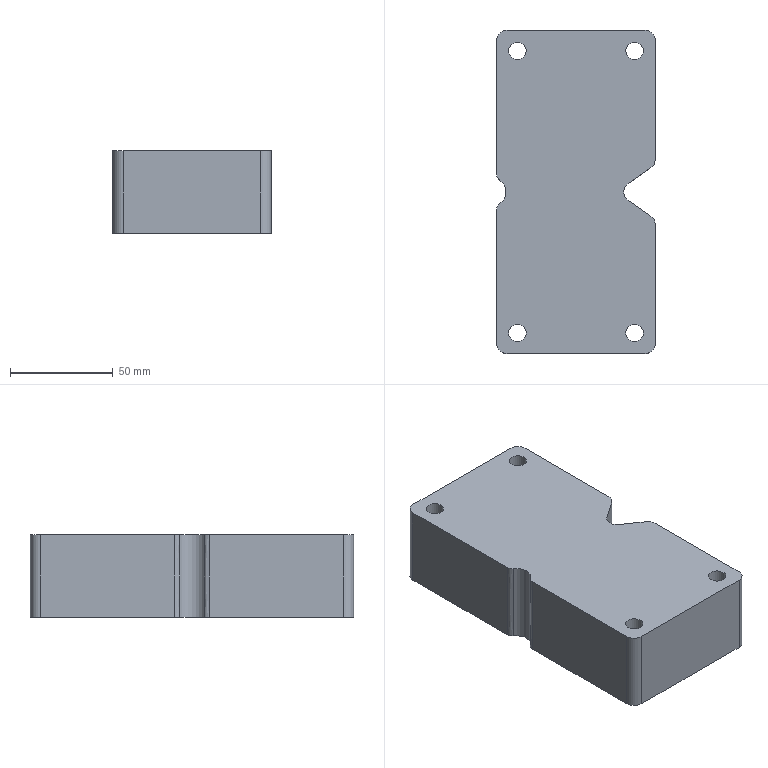Part | NX | features PS-14 2 | 1 solid | 32 faces | box 77 x 157.001 x 40 mm | volume 457397 mm3 | cylinder 16 | plane 14 | spline 2 | commonest cylinder face diameters 10 x7 8.5 x4 14.5 x4 14.05 x1
STEP:
#1=CARTESIAN_POINT('',(2764.236,-866.479,900.716));
#2=VERTEX_POINT('',#1);
#3=CARTESIAN_POINT('',(2764.236,-931.623,900.716));
#4=VERTEX_POINT('',#3);
#5=CARTESIAN_POINT('',(2764.236,-839.123,900.716));
#6=DIRECTION('',(0.,-1.,0.000000114));
#7=VECTOR('',#6,1000.);
#8=LINE('',#5,#7);
#9=EDGE_CURVE('',#2,#4,#8,.T.);
#10=ORIENTED_EDGE('',*,*,#9,.F.);
#11=CARTESIAN_POINT('',(2764.236,-866.479,860.716));
#12=VERTEX_POINT('',#11);
#13=CARTESIAN_POINT('',(2764.236,-866.479,900.716));
#14=CARTESIAN_POINT('',(2764.236,-866.479,887.383));
#15=CARTESIAN_POINT('',(2764.236,-866.479,874.05));
#16=CARTESIAN_POINT('',(2764.236,-866.479,860.716));
#17=B_SPLINE_CURVE_WITH_KNOTS('',3,(#13,#14,#15,#16),.UNSPECIFIED.,.F.,.F.,(4,4),(-0.01,0.03),.UNSPECIFIED.);
#18=EDGE_CURVE('',#2,#12,#17,.T.);
#19=ORIENTED_EDGE('',*,*,#18,.T.);
#20=CARTESIAN_POINT('',(2764.236,-896.605,860.716));
#21=VERTEX_POINT('',#20);
#22=CARTESIAN_POINT('',(2764.236,-839.123,860.716));
#23=DIRECTION('',(0.,1.,-0.000000114));
#24=VECTOR('',#23,1000.);
#25=LINE('',#22,#24);
#26=EDGE_CURVE('',#21,#12,#25,.T.);
#27=ORIENTED_EDGE('',*,*,#26,.F.);
#28=CARTESIAN_POINT('',(2764.236,-931.623,860.716));
#29=VERTEX_POINT('',#28);
#30=CARTESIAN_POINT('',(2764.236,-839.123,860.716));
#31=DIRECTION('',(0.,1.,-0.000000114));
#32=VECTOR('',#31,1000.);
#33=LINE('',#30,#32);
#34=EDGE_CURVE('',#29,#21,#33,.T.);
#35=ORIENTED_EDGE('',*,*,#34,.F.);
#36=CARTESIAN_POINT('',(2764.236,-931.623,935.716));
#37=DIRECTION('',(0.,0.,-1.));
#38=VECTOR('',#37,1000.);
#39=LINE('',#36,#38);
#40=EDGE_CURVE('',#29,#4,#39,.F.);
#41=ORIENTED_EDGE('',*,*,#40,.T.);
#42=EDGE_LOOP('',(#10,#19,#27,#35,#41));
#43=FACE_BOUND('',#42,.T.);
#44=CARTESIAN_POINT('',(2764.236,-839.123,930.716));
#45=DIRECTION('',(-1.,0.,0.));
#46=DIRECTION('',(0.,0.000000114,1.));
#47=AXIS2_PLACEMENT_3D('',#44,#45,#46);
#48=PLANE('',#47);
#49=ADVANCED_FACE('',(#43),#48,.T.);
#50=CARTESIAN_POINT('',(2769.236,-779.622,860.716));
#51=VERTEX_POINT('',#50);
#52=CARTESIAN_POINT('',(2769.236,-779.622,900.716));
#53=VERTEX_POINT('',#52);
#54=CARTESIAN_POINT('',(2769.236,-779.622,935.716));
#55=DIRECTION('',(0.,0.,-1.));
#56=VECTOR('',#55,1000.);
#57=LINE('',#54,#56);
#58=EDGE_CURVE('',#51,#53,#57,.F.);
#59=ORIENTED_EDGE('',*,*,#58,.T.);
#60=CARTESIAN_POINT('',(2836.236,-779.622,900.716));
#61=VERTEX_POINT('',#60);
#62=CARTESIAN_POINT('',(2802.736,-779.622,900.716));
#63=DIRECTION('',(-1.,0.,0.));
#64=VECTOR('',#63,1000.);
#65=LINE('',#62,#64);
#66=EDGE_CURVE('',#61,#53,#65,.T.);
#67=ORIENTED_EDGE('',*,*,#66,.F.);
#68=CARTESIAN_POINT('',(2836.236,-779.622,860.716));
#69=VERTEX_POINT('',#68);
#70=CARTESIAN_POINT('',(2836.236,-779.622,860.716));
#71=DIRECTION('',(0.,0.,-1.));
#72=VECTOR('',#71,1000.);
#73=LINE('',#70,#72);
#74=EDGE_CURVE('',#61,#69,#73,.T.);
#75=ORIENTED_EDGE('',*,*,#74,.T.);
#76=CARTESIAN_POINT('',(2798.548,-779.622,860.716));
#77=VERTEX_POINT('',#76);
#78=CARTESIAN_POINT('',(2765.986,-779.622,860.716));
#79=DIRECTION('',(1.,0.,0.));
#80=VECTOR('',#79,1000.);
#81=LINE('',#78,#80);
#82=EDGE_CURVE('',#77,#69,#81,.T.);
#83=ORIENTED_EDGE('',*,*,#82,.F.);
#84=CARTESIAN_POINT('',(2793.195,-779.622,860.716));
#85=VERTEX_POINT('',#84);
#86=CARTESIAN_POINT('',(2765.986,-779.622,860.716));
#87=DIRECTION('',(1.,0.,0.));
#88=VECTOR('',#87,1000.);
#89=LINE('',#86,#88);
#90=EDGE_CURVE('',#85,#77,#89,.T.);
#91=ORIENTED_EDGE('',*,*,#90,.F.);
#92=CARTESIAN_POINT('',(2765.986,-779.622,860.716));
#93=DIRECTION('',(1.,0.,0.));
#94=VECTOR('',#93,1000.);
#95=LINE('',#92,#94);
#96=EDGE_CURVE('',#51,#85,#95,.T.);
#97=ORIENTED_EDGE('',*,*,#96,.F.);
#98=EDGE_LOOP('',(#59,#67,#75,#83,#91,#97));
#99=FACE_BOUND('',#98,.T.);
#100=CARTESIAN_POINT('',(2765.986,-779.622,841.216));
#101=DIRECTION('',(0.,-1.,0.));
#102=DIRECTION('',(0.,0.,-1.));
#103=AXIS2_PLACEMENT_3D('',#100,#101,#102);
#104=PLANE('',#103);
#105=ADVANCED_FACE('',(#99),#104,.F.);
#106=CARTESIAN_POINT('',(2764.236,-849.765,860.716));
#107=VERTEX_POINT('',#106);
#108=CARTESIAN_POINT('',(2764.236,-819.639,860.716));
#109=VERTEX_POINT('',#108);
#110=CARTESIAN_POINT('',(2764.236,-839.123,860.716));
#111=DIRECTION('',(0.,1.,-0.000000114));
#112=VECTOR('',#111,1000.);
#113=LINE('',#110,#112);
#114=EDGE_CURVE('',#107,#109,#113,.T.);
#115=ORIENTED_EDGE('',*,*,#114,.F.);
#116=CARTESIAN_POINT('',(2764.236,-849.765,900.716));
#117=VERTEX_POINT('',#116);
#118=CARTESIAN_POINT('',(2764.236,-849.765,860.716));
#119=CARTESIAN_POINT('',(2764.236,-849.765,874.05));
#120=CARTESIAN_POINT('',(2764.236,-849.765,887.383));
#121=CARTESIAN_POINT('',(2764.236,-849.765,900.716));
#122=B_SPLINE_CURVE_WITH_KNOTS('',3,(#118,#119,#120,#121),.UNSPECIFIED.,.F.,.F.,(4,4),(0.,0.04),.UNSPECIFIED.);
#123=EDGE_CURVE('',#107,#117,#122,.T.);
#124=ORIENTED_EDGE('',*,*,#123,.T.);
#125=CARTESIAN_POINT('',(2764.236,-784.622,900.716));
#126=VERTEX_POINT('',#125);
#127=CARTESIAN_POINT('',(2764.236,-839.123,900.716));
#128=DIRECTION('',(0.,-1.,0.000000114));
#129=VECTOR('',#128,1000.);
#130=LINE('',#127,#129);
#131=EDGE_CURVE('',#126,#117,#130,.T.);
#132=ORIENTED_EDGE('',*,*,#131,.F.);
#133=CARTESIAN_POINT('',(2764.236,-784.622,860.716));
#134=VERTEX_POINT('',#133);
#135=CARTESIAN_POINT('',(2764.236,-784.622,860.716));
#136=DIRECTION('',(0.,0.,-1.));
#137=VECTOR('',#136,1000.);
#138=LINE('',#135,#137);
#139=EDGE_CURVE('',#126,#134,#138,.T.);
#140=ORIENTED_EDGE('',*,*,#139,.T.);
#141=CARTESIAN_POINT('',(2764.236,-839.123,860.716));
#142=DIRECTION('',(0.,1.,-0.000000114));
#143=VECTOR('',#142,1000.);
#144=LINE('',#141,#143);
#145=EDGE_CURVE('',#109,#134,#144,.T.);
#146=ORIENTED_EDGE('',*,*,#145,.F.);
#147=EDGE_LOOP('',(#115,#124,#132,#140,#146));
#148=FACE_BOUND('',#147,.T.);
#149=CARTESIAN_POINT('',(2764.236,-839.123,930.716));
#150=DIRECTION('',(-1.,0.,0.));
#151=DIRECTION('',(0.,0.000000114,1.));
#152=AXIS2_PLACEMENT_3D('',#149,#150,#151);
#153=PLANE('',#152);
#154=ADVANCED_FACE('',(#148),#153,.T.);
#155=CARTESIAN_POINT('',(2774.236,-782.373,860.716));
#156=VERTEX_POINT('',#155);
#157=CARTESIAN_POINT('',(2774.236,-789.623,860.716));
#158=DIRECTION('',(0.,-0.000000114,-1.));
#159=DIRECTION('',(0.,1.,-0.000000114));
#160=AXIS2_PLACEMENT_3D('',#157,#158,#159);
#161=CIRCLE('',#160,7.25);
#162=EDGE_CURVE('',#156,#156,#161,.T.);
#163=ORIENTED_EDGE('',*,*,#162,.F.);
#164=EDGE_LOOP('',(#163));
#165=FACE_BOUND('',#164,.T.);
#166=CARTESIAN_POINT('',(2831.236,-919.373,860.716));
#167=VERTEX_POINT('',#166);
#168=CARTESIAN_POINT('',(2831.236,-926.623,860.716));
#169=DIRECTION('',(0.,-0.000000114,-1.));
#170=DIRECTION('',(0.,1.,-0.000000114));
#171=AXIS2_PLACEMENT_3D('',#168,#169,#170);
#172=CIRCLE('',#171,7.25);
#173=EDGE_CURVE('',#167,#167,#172,.T.);
#174=ORIENTED_EDGE('',*,*,#173,.F.);
#175=EDGE_LOOP('',(#174));
#176=FACE_BOUND('',#175,.T.);
#177=CARTESIAN_POINT('',(2831.236,-782.373,860.716));
#178=VERTEX_POINT('',#177);
#179=CARTESIAN_POINT('',(2831.236,-789.623,860.716));
#180=DIRECTION('',(0.,-0.000000114,-1.));
#181=DIRECTION('',(0.,1.,-0.000000114));
#182=AXIS2_PLACEMENT_3D('',#179,#180,#181);
#183=CIRCLE('',#182,7.25);
#184=EDGE_CURVE('',#178,#178,#183,.T.);
#185=ORIENTED_EDGE('',*,*,#184,.F.);
#186=EDGE_LOOP('',(#185));
#187=FACE_BOUND('',#186,.T.);
#188=CARTESIAN_POINT('',(2774.236,-919.373,860.716));
#189=VERTEX_POINT('',#188);
#190=CARTESIAN_POINT('',(2774.236,-926.623,860.716));
#191=DIRECTION('',(0.,-0.000000114,-1.));
#192=DIRECTION('',(0.,1.,-0.000000114));
#193=AXIS2_PLACEMENT_3D('',#190,#191,#192);
#194=CIRCLE('',#193,7.25);
#195=EDGE_CURVE('',#189,#189,#194,.T.);
#196=ORIENTED_EDGE('',*,*,#195,.F.);
#197=EDGE_LOOP('',(#196));
#198=FACE_BOUND('',#197,.T.);
#199=ORIENTED_EDGE('',*,*,#26,.T.);
#200=CARTESIAN_POINT('',(2765.579,-863.979,860.716));
#201=VERTEX_POINT('',#200);
#202=CARTESIAN_POINT('',(2767.236,-866.479,860.716));
#203=DIRECTION('',(0.,-0.000000114,-1.));
#204=DIRECTION('',(0.,1.,-0.000000114));
#205=AXIS2_PLACEMENT_3D('',#202,#203,#204);
#206=CIRCLE('',#205,3.);
#207=EDGE_CURVE('',#12,#201,#206,.T.);
#208=ORIENTED_EDGE('',*,*,#207,.T.);
#209=CARTESIAN_POINT('',(2765.579,-852.266,860.716));
#210=VERTEX_POINT('',#209);
#211=CARTESIAN_POINT('',(2761.699,-858.122,860.716));
#212=DIRECTION('',(0.,-0.000000114,-1.));
#213=DIRECTION('',(0.,1.,-0.000000114));
#214=AXIS2_PLACEMENT_3D('',#211,#212,#213);
#215=CIRCLE('',#214,7.025);
#216=EDGE_CURVE('',#201,#210,#215,.F.);
#217=ORIENTED_EDGE('',*,*,#216,.T.);
#218=CARTESIAN_POINT('',(2767.236,-849.765,860.716));
#219=DIRECTION('',(0.,-0.000000114,-1.));
#220=DIRECTION('',(0.,1.,-0.000000114));
#221=AXIS2_PLACEMENT_3D('',#218,#219,#220);
#222=CIRCLE('',#221,3.);
#223=EDGE_CURVE('',#210,#107,#222,.T.);
#224=ORIENTED_EDGE('',*,*,#223,.T.);
#225=ORIENTED_EDGE('',*,*,#114,.T.);
#226=ORIENTED_EDGE('',*,*,#145,.T.);
#227=CARTESIAN_POINT('',(2769.236,-784.622,860.716));
#228=DIRECTION('',(0.,-0.000000114,-1.));
#229=DIRECTION('',(0.,1.,-0.000000114));
#230=AXIS2_PLACEMENT_3D('',#227,#228,#229);
#231=CIRCLE('',#230,5.);
#232=EDGE_CURVE('',#134,#51,#231,.T.);
#233=ORIENTED_EDGE('',*,*,#232,.T.);
#234=ORIENTED_EDGE('',*,*,#96,.T.);
#235=ORIENTED_EDGE('',*,*,#90,.T.);
#236=ORIENTED_EDGE('',*,*,#82,.T.);
#237=CARTESIAN_POINT('',(2841.236,-784.622,860.716));
#238=VERTEX_POINT('',#237);
#239=CARTESIAN_POINT('',(2836.236,-784.622,860.716));
#240=DIRECTION('',(0.,-0.000000114,-1.));
#241=DIRECTION('',(0.,1.,-0.000000114));
#242=AXIS2_PLACEMENT_3D('',#239,#240,#241);
#243=CIRCLE('',#242,5.);
#244=EDGE_CURVE('',#69,#238,#243,.T.);
#245=ORIENTED_EDGE('',*,*,#244,.T.);
#246=CARTESIAN_POINT('',(2841.236,-842.26,860.716));
#247=VERTEX_POINT('',#246);
#248=CARTESIAN_POINT('',(2841.236,-839.123,860.716));
#249=DIRECTION('',(0.,-1.,0.000000114));
#250=VECTOR('',#249,1000.);
#251=LINE('',#248,#250);
#252=EDGE_CURVE('',#238,#247,#251,.T.);
#253=ORIENTED_EDGE('',*,*,#252,.T.);
#254=CARTESIAN_POINT('',(2839.088,-846.366,860.716));
#255=VERTEX_POINT('',#254);
#256=CARTESIAN_POINT('',(2836.236,-842.26,860.716));
#257=DIRECTION('',(0.,-0.000000114,-1.));
#258=DIRECTION('',(0.,1.,-0.000000114));
#259=AXIS2_PLACEMENT_3D('',#256,#257,#258);
#260=CIRCLE('',#259,5.);
#261=EDGE_CURVE('',#247,#255,#260,.T.);
#262=ORIENTED_EDGE('',*,*,#261,.T.);
#263=CARTESIAN_POINT('',(2828.076,-854.015,860.716));
#264=VERTEX_POINT('',#263);
#265=CARTESIAN_POINT('',(2824.687,-856.37,860.716));
#266=DIRECTION('',(0.8213,0.5705,-0.000000065));
#267=VECTOR('',#266,1000.);
#268=LINE('',#265,#267);
#269=EDGE_CURVE('',#264,#255,#268,.T.);
#270=ORIENTED_EDGE('',*,*,#269,.F.);
#271=CARTESIAN_POINT('',(2828.076,-862.229,860.716));
#272=VERTEX_POINT('',#271);
#273=CARTESIAN_POINT('',(2830.929,-858.122,860.716));
#274=DIRECTION('',(0.,-0.000000114,-1.));
#275=DIRECTION('',(0.,1.,-0.000000114));
#276=AXIS2_PLACEMENT_3D('',#273,#274,#275);
#277=CIRCLE('',#276,5.);
#278=EDGE_CURVE('',#264,#272,#277,.F.);
#279=ORIENTED_EDGE('',*,*,#278,.T.);
#280=CARTESIAN_POINT('',(2839.088,-869.878,860.716));
#281=VERTEX_POINT('',#280);
#282=CARTESIAN_POINT('',(2830.595,-863.978,860.716));
#283=DIRECTION('',(0.8213,-0.5705,0.000000065));
#284=VECTOR('',#283,1000.);
#285=LINE('',#282,#284);
#286=EDGE_CURVE('',#272,#281,#285,.T.);
#287=ORIENTED_EDGE('',*,*,#286,.T.);
#288=CARTESIAN_POINT('',(2841.236,-873.984,860.716));
#289=VERTEX_POINT('',#288);
#290=CARTESIAN_POINT('',(2836.236,-873.984,860.716));
#291=DIRECTION('',(0.,-0.000000114,-1.));
#292=DIRECTION('',(0.,1.,-0.000000114));
#293=AXIS2_PLACEMENT_3D('',#290,#291,#292);
#294=CIRCLE('',#293,5.);
#295=EDGE_CURVE('',#281,#289,#294,.T.);
#296=ORIENTED_EDGE('',*,*,#295,.T.);
#297=CARTESIAN_POINT('',(2841.236,-931.623,860.716));
#298=VERTEX_POINT('',#297);
#299=CARTESIAN_POINT('',(2841.236,-839.123,860.716));
#300=DIRECTION('',(0.,-1.,0.000000114));
#301=VECTOR('',#300,1000.);
#302=LINE('',#299,#301);
#303=EDGE_CURVE('',#289,#298,#302,.T.);
#304=ORIENTED_EDGE('',*,*,#303,.T.);
#305=CARTESIAN_POINT('',(2836.236,-936.623,860.716));
#306=VERTEX_POINT('',#305);
#307=CARTESIAN_POINT('',(2836.236,-931.623,860.716));
#308=DIRECTION('',(0.,-0.000000114,-1.));
#309=DIRECTION('',(0.,1.,-0.000000114));
#310=AXIS2_PLACEMENT_3D('',#307,#308,#309);
#311=CIRCLE('',#310,5.);
#312=EDGE_CURVE('',#298,#306,#311,.T.);
#313=ORIENTED_EDGE('',*,*,#312,.T.);
#314=CARTESIAN_POINT('',(2798.548,-936.623,860.716));
#315=VERTEX_POINT('',#314);
#316=CARTESIAN_POINT('',(2812.707,-936.623,860.716));
#317=DIRECTION('',(1.,0.,0.));
#318=VECTOR('',#317,1000.);
#319=LINE('',#316,#318);
#320=EDGE_CURVE('',#315,#306,#319,.T.);
#321=ORIENTED_EDGE('',*,*,#320,.F.);
#322=CARTESIAN_POINT('',(2793.195,-936.623,860.716));
#323=VERTEX_POINT('',#322);
#324=CARTESIAN_POINT('',(2812.707,-936.623,860.716));
#325=DIRECTION('',(1.,0.,0.));
#326=VECTOR('',#325,1000.);
#327=LINE('',#324,#326);
#328=EDGE_CURVE('',#323,#315,#327,.T.);
#329=ORIENTED_EDGE('',*,*,#328,.F.);
#330=CARTESIAN_POINT('',(2769.236,-936.623,860.716));
#331=VERTEX_POINT('',#330);
#332=CARTESIAN_POINT('',(2812.707,-936.623,860.716));
#333=DIRECTION('',(1.,0.,0.));
#334=VECTOR('',#333,1000.);
#335=LINE('',#332,#334);
#336=EDGE_CURVE('',#331,#323,#335,.T.);
#337=ORIENTED_EDGE('',*,*,#336,.F.);
#338=CARTESIAN_POINT('',(2769.236,-931.623,860.716));
#339=DIRECTION('',(0.,-0.000000114,-1.));
#340=DIRECTION('',(0.,1.,-0.000000114));
#341=AXIS2_PLACEMENT_3D('',#338,#339,#340);
#342=CIRCLE('',#341,5.);
#343=EDGE_CURVE('',#331,#29,#342,.T.);
#344=ORIENTED_EDGE('',*,*,#343,.T.);
#345=ORIENTED_EDGE('',*,*,#34,.T.);
#346=EDGE_LOOP('',(#199,#208,#217,#224,#225,#226,#233,#234,#235,#236,#245,#253,#262,#270,#279,#287,#296,#304,#313,#321,#329,#337,#344,#345));
#347=FACE_BOUND('',#346,.T.);
#348=CARTESIAN_POINT('',(2812.707,-839.123,860.716));
#349=DIRECTION('',(0.,-0.000000114,-1.));
#350=DIRECTION('',(0.,-1.,0.000000114));
#351=AXIS2_PLACEMENT_3D('',#348,#349,#350);
#352=PLANE('',#351);
#353=ADVANCED_FACE('',(#165,#176,#187,#198,#347),#352,.T.);
#354=CARTESIAN_POINT('',(2841.236,-842.26,900.716));
#355=VERTEX_POINT('',#354);
#356=CARTESIAN_POINT('',(2841.236,-784.622,900.716));
#357=VERTEX_POINT('',#356);
#358=CARTESIAN_POINT('',(2841.236,-838.813,900.716));
#359=DIRECTION('',(0.,1.,-0.000000114));
#360=VECTOR('',#359,1000.);
#361=LINE('',#358,#360);
#362=EDGE_CURVE('',#355,#357,#361,.T.);
#363=ORIENTED_EDGE('',*,*,#362,.F.);
#364=CARTESIAN_POINT('',(2841.236,-842.26,860.716));
#365=DIRECTION('',(0.,0.,-1.));
#366=VECTOR('',#365,1000.);
#367=LINE('',#364,#366);
#368=EDGE_CURVE('',#355,#247,#367,.T.);
#369=ORIENTED_EDGE('',*,*,#368,.T.);
#370=ORIENTED_EDGE('',*,*,#252,.F.);
#371=CARTESIAN_POINT('',(2841.236,-784.622,935.716));
#372=DIRECTION('',(0.,0.,-1.));
#373=VECTOR('',#372,1000.);
#374=LINE('',#371,#373);
#375=EDGE_CURVE('',#238,#357,#374,.F.);
#376=ORIENTED_EDGE('',*,*,#375,.T.);
#377=EDGE_LOOP('',(#363,#369,#370,#376));
#378=FACE_BOUND('',#377,.T.);
#379=CARTESIAN_POINT('',(2841.236,-838.813,930.716));
#380=DIRECTION('',(1.,0.,0.));
#381=DIRECTION('',(0.,-0.000000114,-1.));
#382=AXIS2_PLACEMENT_3D('',#379,#380,#381);
#383=PLANE('',#382);
#384=ADVANCED_FACE('',(#378),#383,.T.);
#385=CARTESIAN_POINT('',(2839.088,-846.366,900.716));
#386=VERTEX_POINT('',#385);
#387=CARTESIAN_POINT('',(2839.088,-846.366,935.716));
#388=DIRECTION('',(0.,0.,-1.));
#389=VECTOR('',#388,1000.);
#390=LINE('',#387,#389);
#391=EDGE_CURVE('',#255,#386,#390,.F.);
#392=ORIENTED_EDGE('',*,*,#391,.T.);
#393=CARTESIAN_POINT('',(2828.076,-854.015,900.716));
#394=VERTEX_POINT('',#393);
#395=CARTESIAN_POINT('',(2830.599,-852.263,900.716));
#396=DIRECTION('',(-0.8213,-0.5705,0.000000065));
#397=VECTOR('',#396,1000.);
#398=LINE('',#395,#397);
#399=EDGE_CURVE('',#386,#394,#398,.T.);
#400=ORIENTED_EDGE('',*,*,#399,.T.);
#401=CARTESIAN_POINT('',(2828.076,-854.015,859.72));
#402=DIRECTION('',(0.,0.,-1.));
#403=VECTOR('',#402,1000.);
#404=LINE('',#401,#403);
#405=EDGE_CURVE('',#394,#264,#404,.T.);
#406=ORIENTED_EDGE('',*,*,#405,.T.);
#407=ORIENTED_EDGE('',*,*,#269,.T.);
#408=EDGE_LOOP('',(#392,#400,#406,#407));
#409=FACE_BOUND('',#408,.T.);
#410=CARTESIAN_POINT('',(2830.599,-852.263,859.716));
#411=DIRECTION('',(-0.5705,0.8213,0.));
#412=DIRECTION('',(-0.8213,-0.5705,0.));
#413=AXIS2_PLACEMENT_3D('',#410,#411,#412);
#414=PLANE('',#413);
#415=ADVANCED_FACE('',(#409),#414,.F.);
#416=CARTESIAN_POINT('',(2828.076,-862.229,900.716));
#417=VERTEX_POINT('',#416);
#418=CARTESIAN_POINT('',(2828.076,-862.229,859.72));
#419=DIRECTION('',(0.,0.,-1.));
#420=VECTOR('',#419,1000.);
#421=LINE('',#418,#420);
#422=EDGE_CURVE('',#272,#417,#421,.F.);
#423=ORIENTED_EDGE('',*,*,#422,.T.);
#424=CARTESIAN_POINT('',(2839.088,-869.878,900.716));
#425=VERTEX_POINT('',#424);
#426=CARTESIAN_POINT('',(2809.059,-849.019,900.716));
#427=DIRECTION('',(-0.8213,0.5705,-0.000000065));
#428=VECTOR('',#427,1000.);
#429=LINE('',#426,#428);
#430=EDGE_CURVE('',#425,#417,#429,.T.);
#431=ORIENTED_EDGE('',*,*,#430,.F.);
#432=CARTESIAN_POINT('',(2839.088,-869.878,860.716));
#433=DIRECTION('',(0.,0.,1.));
#434=VECTOR('',#433,1000.);
#435=LINE('',#432,#434);
#436=EDGE_CURVE('',#425,#281,#435,.F.);
#437=ORIENTED_EDGE('',*,*,#436,.T.);
#438=ORIENTED_EDGE('',*,*,#286,.F.);
#439=EDGE_LOOP('',(#423,#431,#437,#438));
#440=FACE_BOUND('',#439,.T.);
#441=CARTESIAN_POINT('',(2830.595,-863.978,859.72));
#442=DIRECTION('',(-0.5705,-0.8213,0.));
#443=DIRECTION('',(0.8213,-0.5705,0.));
#444=AXIS2_PLACEMENT_3D('',#441,#442,#443);
#445=PLANE('',#444);
#446=ADVANCED_FACE('',(#440),#445,.F.);
#447=CARTESIAN_POINT('',(2841.236,-873.984,900.716));
#448=VERTEX_POINT('',#447);
#449=CARTESIAN_POINT('',(2841.236,-931.623,900.716));
#450=VERTEX_POINT('',#449);
#451=CARTESIAN_POINT('',(2841.236,-858.122,900.716));
#452=DIRECTION('',(0.,-1.,0.000000114));
#453=VECTOR('',#452,1000.);
#454=LINE('',#451,#453);
#455=EDGE_CURVE('',#448,#450,#454,.T.);
#456=ORIENTED_EDGE('',*,*,#455,.T.);
#457=CARTESIAN_POINT('',(2841.236,-931.623,860.716));
#458=DIRECTION('',(0.,0.,1.));
#459=VECTOR('',#458,1000.);
#460=LINE('',#457,#459);
#461=EDGE_CURVE('',#450,#298,#460,.F.);
#462=ORIENTED_EDGE('',*,*,#461,.T.);
#463=ORIENTED_EDGE('',*,*,#303,.F.);
#464=CARTESIAN_POINT('',(2841.236,-873.984,935.716));
#465=DIRECTION('',(0.,0.,1.));
#466=VECTOR('',#465,1000.);
#467=LINE('',#464,#466);
#468=EDGE_CURVE('',#289,#448,#467,.T.);
#469=ORIENTED_EDGE('',*,*,#468,.T.);
#470=EDGE_LOOP('',(#456,#462,#463,#469));
#471=FACE_BOUND('',#470,.T.);
#472=CARTESIAN_POINT('',(2841.236,-838.813,930.716));
#473=DIRECTION('',(1.,0.,0.));
#474=DIRECTION('',(0.,-0.000000114,-1.));
#475=AXIS2_PLACEMENT_3D('',#472,#473,#474);
#476=PLANE('',#475);
#477=ADVANCED_FACE('',(#471),#476,.T.);
#478=CARTESIAN_POINT('',(2836.236,-936.623,900.716));
#479=VERTEX_POINT('',#478);
#480=CARTESIAN_POINT('',(2836.236,-936.623,935.716));
#481=DIRECTION('',(0.,0.,1.));
#482=VECTOR('',#481,1000.);
#483=LINE('',#480,#482);
#484=EDGE_CURVE('',#306,#479,#483,.T.);
#485=ORIENTED_EDGE('',*,*,#484,.T.);
#486=CARTESIAN_POINT('',(2769.236,-936.623,900.716));
#487=VERTEX_POINT('',#486);
#488=CARTESIAN_POINT('',(2802.736,-936.623,900.716));
#489=DIRECTION('',(1.,0.,0.));
#490=VECTOR('',#489,1000.);
#491=LINE('',#488,#490);
#492=EDGE_CURVE('',#487,#479,#491,.T.);
#493=ORIENTED_EDGE('',*,*,#492,.F.);
#494=CARTESIAN_POINT('',(2769.236,-936.623,860.716));
#495=DIRECTION('',(0.,0.,-1.));
#496=VECTOR('',#495,1000.);
#497=LINE('',#494,#496);
#498=EDGE_CURVE('',#487,#331,#497,.T.);
#499=ORIENTED_EDGE('',*,*,#498,.T.);
#500=ORIENTED_EDGE('',*,*,#336,.T.);
#501=ORIENTED_EDGE('',*,*,#328,.T.);
#502=ORIENTED_EDGE('',*,*,#320,.T.);
#503=EDGE_LOOP('',(#485,#493,#499,#500,#501,#502));
#504=FACE_BOUND('',#503,.T.);
#505=CARTESIAN_POINT('',(2765.986,-936.623,841.216));
#506=DIRECTION('',(0.,1.,0.));
#507=DIRECTION('',(0.,0.,-1.));
#508=AXIS2_PLACEMENT_3D('',#505,#506,#507);
#509=PLANE('',#508);
#510=ADVANCED_FACE('',(#504),#509,.F.);
#511=ORIENTED_EDGE('',*,*,#405,.F.);
#512=CARTESIAN_POINT('',(2830.929,-858.122,900.716));
#513=DIRECTION('',(0.,-0.000000114,-1.));
#514=DIRECTION('',(0.,1.,-0.000000114));
#515=AXIS2_PLACEMENT_3D('',#512,#513,#514);
#516=CIRCLE('',#515,5.);
#517=EDGE_CURVE('',#417,#394,#516,.T.);
#518=ORIENTED_EDGE('',*,*,#517,.F.);
#519=ORIENTED_EDGE('',*,*,#422,.F.);
#520=ORIENTED_EDGE('',*,*,#278,.F.);
#521=EDGE_LOOP('',(#511,#518,#519,#520));
#522=FACE_BOUND('',#521,.T.);
#523=CARTESIAN_POINT('',(2830.929,-858.122,859.72));
#524=DIRECTION('',(0.,0.,-1.));
#525=DIRECTION('',(-1.,0.,0.));
#526=AXIS2_PLACEMENT_3D('',#523,#524,#525);
#527=CYLINDRICAL_SURFACE('',#526,5.);
#528=ADVANCED_FACE('',(#522),#527,.F.);
#529=CARTESIAN_POINT('',(2836.236,-784.622,900.716));
#530=DIRECTION('',(0.,-0.000000114,-1.));
#531=DIRECTION('',(0.,1.,-0.000000114));
#532=AXIS2_PLACEMENT_3D('',#529,#530,#531);
#533=CIRCLE('',#532,5.);
#534=EDGE_CURVE('',#61,#357,#533,.T.);
#535=ORIENTED_EDGE('',*,*,#534,.T.);
#536=ORIENTED_EDGE('',*,*,#375,.F.);
#537=ORIENTED_EDGE('',*,*,#244,.F.);
#538=ORIENTED_EDGE('',*,*,#74,.F.);
#539=EDGE_LOOP('',(#535,#536,#537,#538));
#540=FACE_BOUND('',#539,.T.);
#541=CARTESIAN_POINT('',(2836.236,-784.622,841.216));
#542=DIRECTION('',(0.,0.,1.));
#543=DIRECTION('',(1.,0.,0.));
#544=AXIS2_PLACEMENT_3D('',#541,#542,#543);
#545=CYLINDRICAL_SURFACE('',#544,5.);
#546=ADVANCED_FACE('',(#540),#545,.T.);
#547=CARTESIAN_POINT('',(2836.236,-842.26,900.716));
#548=DIRECTION('',(0.,-0.000000114,-1.));
#549=DIRECTION('',(0.,1.,-0.000000114));
#550=AXIS2_PLACEMENT_3D('',#547,#548,#549);
#551=CIRCLE('',#550,5.);
#552=EDGE_CURVE('',#386,#355,#551,.F.);
#553=ORIENTED_EDGE('',*,*,#552,.F.);
#554=ORIENTED_EDGE('',*,*,#391,.F.);
#555=ORIENTED_EDGE('',*,*,#261,.F.);
#556=ORIENTED_EDGE('',*,*,#368,.F.);
#557=EDGE_LOOP('',(#553,#554,#555,#556));
#558=FACE_BOUND('',#557,.T.);
#559=CARTESIAN_POINT('',(2836.236,-842.26,930.716));
#560=DIRECTION('',(0.,0.,1.));
#561=DIRECTION('',(1.,0.,0.));
#562=AXIS2_PLACEMENT_3D('',#559,#560,#561);
#563=CYLINDRICAL_SURFACE('',#562,5.);
#564=ADVANCED_FACE('',(#558),#563,.T.);
#565=CARTESIAN_POINT('',(2836.236,-873.984,900.716));
#566=DIRECTION('',(0.,-0.000000114,-1.));
#567=DIRECTION('',(0.,1.,-0.000000114));
#568=AXIS2_PLACEMENT_3D('',#565,#566,#567);
#569=CIRCLE('',#568,5.);
#570=EDGE_CURVE('',#448,#425,#569,.F.);
#571=ORIENTED_EDGE('',*,*,#570,.F.);
#572=ORIENTED_EDGE('',*,*,#468,.F.);
#573=ORIENTED_EDGE('',*,*,#295,.F.);
#574=ORIENTED_EDGE('',*,*,#436,.F.);
#575=EDGE_LOOP('',(#571,#572,#573,#574));
#576=FACE_BOUND('',#575,.T.);
#577=CARTESIAN_POINT('',(2836.236,-873.984,930.716));
#578=DIRECTION('',(0.,0.,-1.));
#579=DIRECTION('',(-1.,0.,0.));
#580=AXIS2_PLACEMENT_3D('',#577,#578,#579);
#581=CYLINDRICAL_SURFACE('',#580,5.);
#582=ADVANCED_FACE('',(#576),#581,.T.);
#583=CARTESIAN_POINT('',(2836.236,-931.623,900.716));
#584=DIRECTION('',(0.,-0.000000114,-1.));
#585=DIRECTION('',(0.,1.,-0.000000114));
#586=AXIS2_PLACEMENT_3D('',#583,#584,#585);
#587=CIRCLE('',#586,5.);
#588=EDGE_CURVE('',#479,#450,#587,.F.);
#589=ORIENTED_EDGE('',*,*,#588,.F.);
#590=ORIENTED_EDGE('',*,*,#484,.F.);
#591=ORIENTED_EDGE('',*,*,#312,.F.);
#592=ORIENTED_EDGE('',*,*,#461,.F.);
#593=EDGE_LOOP('',(#589,#590,#591,#592));
#594=FACE_BOUND('',#593,.T.);
#595=CARTESIAN_POINT('',(2836.236,-931.623,841.216));
#596=DIRECTION('',(0.,0.,-1.));
#597=DIRECTION('',(-1.,0.,0.));
#598=AXIS2_PLACEMENT_3D('',#595,#596,#597);
#599=CYLINDRICAL_SURFACE('',#598,5.);
#600=ADVANCED_FACE('',(#594),#599,.T.);
#601=CARTESIAN_POINT('',(2769.236,-784.622,900.716));
#602=DIRECTION('',(0.,-0.000000114,-1.));
#603=DIRECTION('',(0.,1.,-0.000000114));
#604=AXIS2_PLACEMENT_3D('',#601,#602,#603);
#605=CIRCLE('',#604,5.);
#606=EDGE_CURVE('',#53,#126,#605,.F.);
#607=ORIENTED_EDGE('',*,*,#606,.F.);
#608=ORIENTED_EDGE('',*,*,#58,.F.);
#609=ORIENTED_EDGE('',*,*,#232,.F.);
#610=ORIENTED_EDGE('',*,*,#139,.F.);
#611=EDGE_LOOP('',(#607,#608,#609,#610));
#612=FACE_BOUND('',#611,.T.);
#613=CARTESIAN_POINT('',(2769.236,-784.622,930.716));
#614=DIRECTION('',(0.,0.,1.));
#615=DIRECTION('',(1.,0.,0.));
#616=AXIS2_PLACEMENT_3D('',#613,#614,#615);
#617=CYLINDRICAL_SURFACE('',#616,5.);
#618=ADVANCED_FACE('',(#612),#617,.T.);
#619=CARTESIAN_POINT('',(2769.236,-931.623,900.716));
#620=DIRECTION('',(0.,-0.000000114,-1.));
#621=DIRECTION('',(0.,1.,-0.000000114));
#622=AXIS2_PLACEMENT_3D('',#619,#620,#621);
#623=CIRCLE('',#622,5.);
#624=EDGE_CURVE('',#4,#487,#623,.F.);
#625=ORIENTED_EDGE('',*,*,#624,.F.);
#626=ORIENTED_EDGE('',*,*,#40,.F.);
#627=ORIENTED_EDGE('',*,*,#343,.F.);
#628=ORIENTED_EDGE('',*,*,#498,.F.);
#629=EDGE_LOOP('',(#625,#626,#627,#628));
#630=FACE_BOUND('',#629,.T.);
#631=CARTESIAN_POINT('',(2769.236,-931.623,841.216));
#632=DIRECTION('',(0.,0.,1.));
#633=DIRECTION('',(1.,0.,0.));
#634=AXIS2_PLACEMENT_3D('',#631,#632,#633);
#635=CYLINDRICAL_SURFACE('',#634,5.);
#636=ADVANCED_FACE('',(#630),#635,.T.);
#637=CARTESIAN_POINT('',(2774.236,-785.373,900.716));
#638=VERTEX_POINT('',#637);
#639=CARTESIAN_POINT('',(2774.236,-789.623,900.716));
#640=DIRECTION('',(0.,-0.000000114,-1.));
#641=DIRECTION('',(0.,1.,-0.000000114));
#642=AXIS2_PLACEMENT_3D('',#639,#640,#641);
#643=CIRCLE('',#642,4.25);
#644=EDGE_CURVE('',#638,#638,#643,.T.);
#645=ORIENTED_EDGE('',*,*,#644,.T.);
#646=EDGE_LOOP('',(#645));
#647=FACE_BOUND('',#646,.T.);
#648=CARTESIAN_POINT('',(2831.236,-922.373,900.716));
#649=VERTEX_POINT('',#648);
#650=CARTESIAN_POINT('',(2831.236,-926.623,900.716));
#651=DIRECTION('',(0.,-0.000000114,-1.));
#652=DIRECTION('',(0.,1.,-0.000000114));
#653=AXIS2_PLACEMENT_3D('',#650,#651,#652);
#654=CIRCLE('',#653,4.25);
#655=EDGE_CURVE('',#649,#649,#654,.T.);
#656=ORIENTED_EDGE('',*,*,#655,.T.);
#657=EDGE_LOOP('',(#656));
#658=FACE_BOUND('',#657,.T.);
#659=CARTESIAN_POINT('',(2831.236,-785.373,900.716));
#660=VERTEX_POINT('',#659);
#661=CARTESIAN_POINT('',(2831.236,-789.623,900.716));
#662=DIRECTION('',(0.,-0.000000114,-1.));
#663=DIRECTION('',(0.,1.,-0.000000114));
#664=AXIS2_PLACEMENT_3D('',#661,#662,#663);
#665=CIRCLE('',#664,4.25);
#666=EDGE_CURVE('',#660,#660,#665,.T.);
#667=ORIENTED_EDGE('',*,*,#666,.T.);
#668=EDGE_LOOP('',(#667));
#669=FACE_BOUND('',#668,.T.);
#670=CARTESIAN_POINT('',(2774.236,-922.373,900.716));
#671=VERTEX_POINT('',#670);
#672=CARTESIAN_POINT('',(2774.236,-926.623,900.716));
#673=DIRECTION('',(0.,-0.000000114,-1.));
#674=DIRECTION('',(0.,1.,-0.000000114));
#675=AXIS2_PLACEMENT_3D('',#672,#673,#674);
#676=CIRCLE('',#675,4.25);
#677=EDGE_CURVE('',#671,#671,#676,.T.);
#678=ORIENTED_EDGE('',*,*,#677,.T.);
#679=EDGE_LOOP('',(#678));
#680=FACE_BOUND('',#679,.T.);
#681=CARTESIAN_POINT('',(2765.579,-852.266,900.716));
#682=VERTEX_POINT('',#681);
#683=CARTESIAN_POINT('',(2765.579,-863.979,900.716));
#684=VERTEX_POINT('',#683);
#685=CARTESIAN_POINT('',(2761.699,-858.122,900.716));
#686=DIRECTION('',(0.,-0.000000114,-1.));
#687=DIRECTION('',(0.,1.,-0.000000114));
#688=AXIS2_PLACEMENT_3D('',#685,#686,#687);
#689=CIRCLE('',#688,7.025);
#690=EDGE_CURVE('',#682,#684,#689,.T.);
#691=ORIENTED_EDGE('',*,*,#690,.T.);
#692=CARTESIAN_POINT('',(2767.236,-866.479,900.716));
#693=DIRECTION('',(0.,-0.000000114,-1.));
#694=DIRECTION('',(0.,1.,-0.000000114));
#695=AXIS2_PLACEMENT_3D('',#692,#693,#694);
#696=CIRCLE('',#695,3.);
#697=EDGE_CURVE('',#684,#2,#696,.F.);
#698=ORIENTED_EDGE('',*,*,#697,.T.);
#699=ORIENTED_EDGE('',*,*,#9,.T.);
#700=ORIENTED_EDGE('',*,*,#624,.T.);
#701=ORIENTED_EDGE('',*,*,#492,.T.);
#702=ORIENTED_EDGE('',*,*,#588,.T.);
#703=ORIENTED_EDGE('',*,*,#455,.F.);
#704=ORIENTED_EDGE('',*,*,#570,.T.);
#705=ORIENTED_EDGE('',*,*,#430,.T.);
#706=ORIENTED_EDGE('',*,*,#517,.T.);
#707=ORIENTED_EDGE('',*,*,#399,.F.);
#708=ORIENTED_EDGE('',*,*,#552,.T.);
#709=ORIENTED_EDGE('',*,*,#362,.T.);
#710=ORIENTED_EDGE('',*,*,#534,.F.);
#711=ORIENTED_EDGE('',*,*,#66,.T.);
#712=ORIENTED_EDGE('',*,*,#606,.T.);
#713=ORIENTED_EDGE('',*,*,#131,.T.);
#714=CARTESIAN_POINT('',(2767.236,-849.765,900.716));
#715=DIRECTION('',(0.,-0.000000114,-1.));
#716=DIRECTION('',(0.,1.,-0.000000114));
#717=AXIS2_PLACEMENT_3D('',#714,#715,#716);
#718=CIRCLE('',#717,3.);
#719=EDGE_CURVE('',#117,#682,#718,.F.);
#720=ORIENTED_EDGE('',*,*,#719,.T.);
#721=EDGE_LOOP('',(#691,#698,#699,#700,#701,#702,#703,#704,#705,#706,#707,#708,#709,#710,#711,#712,#713,#720));
#722=FACE_BOUND('',#721,.T.);
#723=CARTESIAN_POINT('',(2802.736,-858.122,900.716));
#724=DIRECTION('',(0.,-0.000000114,-1.));
#725=DIRECTION('',(0.,1.,-0.000000114));
#726=AXIS2_PLACEMENT_3D('',#723,#724,#725);
#727=PLANE('',#726);
#728=ADVANCED_FACE('',(#647,#658,#669,#680,#722),#727,.F.);
#729=ORIENTED_EDGE('',*,*,#216,.F.);
#730=CARTESIAN_POINT('',(2765.579,-863.979,860.716));
#731=CARTESIAN_POINT('',(2765.579,-863.979,874.05));
#732=CARTESIAN_POINT('',(2765.579,-863.979,887.383));
#733=CARTESIAN_POINT('',(2765.579,-863.979,900.716));
#734=B_SPLINE_CURVE_WITH_KNOTS('',3,(#730,#731,#732,#733),.UNSPECIFIED.,.F.,.F.,(4,4),(0.,0.04),.UNSPECIFIED.);
#735=EDGE_CURVE('',#201,#684,#734,.T.);
#736=ORIENTED_EDGE('',*,*,#735,.T.);
#737=ORIENTED_EDGE('',*,*,#690,.F.);
#738=CARTESIAN_POINT('',(2765.579,-852.266,900.716));
#739=CARTESIAN_POINT('',(2765.579,-852.266,887.383));
#740=CARTESIAN_POINT('',(2765.579,-852.266,874.05));
#741=CARTESIAN_POINT('',(2765.579,-852.266,860.716));
#742=B_SPLINE_CURVE_WITH_KNOTS('',3,(#738,#739,#740,#741),.UNSPECIFIED.,.F.,.F.,(4,4),(-0.01,0.03),.UNSPECIFIED.);
#743=EDGE_CURVE('',#682,#210,#742,.T.);
#744=ORIENTED_EDGE('',*,*,#743,.T.);
#745=EDGE_LOOP('',(#729,#736,#737,#744));
#746=FACE_BOUND('',#745,.T.);
#747=CARTESIAN_POINT('',(2761.699,-858.122,858.716));
#748=DIRECTION('',(0.,0.,1.));
#749=DIRECTION('',(1.,0.,0.));
#750=AXIS2_PLACEMENT_3D('',#747,#748,#749);
#751=CYLINDRICAL_SURFACE('',#750,7.025);
#752=ADVANCED_FACE('',(#746),#751,.F.);
#753=ORIENTED_EDGE('',*,*,#207,.F.);
#754=ORIENTED_EDGE('',*,*,#18,.F.);
#755=ORIENTED_EDGE('',*,*,#697,.F.);
#756=ORIENTED_EDGE('',*,*,#735,.F.);
#757=EDGE_LOOP('',(#753,#754,#755,#756));
#758=FACE_BOUND('',#757,.T.);
#759=CARTESIAN_POINT('',(2765.579,-863.979,900.716));
#760=CARTESIAN_POINT('',(2764.236,-864.868,900.716));
#761=CARTESIAN_POINT('',(2764.236,-866.479,900.716));
#762=CARTESIAN_POINT('',(2765.579,-863.979,887.383));
#763=CARTESIAN_POINT('',(2764.236,-864.868,887.383));
#764=CARTESIAN_POINT('',(2764.236,-866.479,887.383));
#765=CARTESIAN_POINT('',(2765.579,-863.979,874.05));
#766=CARTESIAN_POINT('',(2764.236,-864.868,874.05));
#767=CARTESIAN_POINT('',(2764.236,-866.479,874.05));
#768=CARTESIAN_POINT('',(2765.579,-863.979,860.716));
#769=CARTESIAN_POINT('',(2764.236,-864.868,860.716));
#770=CARTESIAN_POINT('',(2764.236,-866.479,860.716));
#771=(BOUNDED_SURFACE()B_SPLINE_SURFACE(3,2,((#759,#760,#761),(#762,#763,#764),(#765,#766,#767),(#768,#769,#770)),.UNSPECIFIED.,.F.,.F.,.F.)B_SPLINE_SURFACE_WITH_KNOTS((4,4),(3,3),(0.07617,0.1162),(0.,1.),.PIECEWISE_BEZIER_KNOTS.)GEOMETRIC_REPRESENTATION_ITEM()RATIONAL_B_SPLINE_SURFACE(((1.,0.881,1.),(1.,0.881,1.),(1.,0.881,1.),(1.,0.881,1.)))REPRESENTATION_ITEM('')SURFACE());
#772=ADVANCED_FACE('',(#758),#771,.T.);
#773=ORIENTED_EDGE('',*,*,#719,.F.);
#774=ORIENTED_EDGE('',*,*,#123,.F.);
#775=ORIENTED_EDGE('',*,*,#223,.F.);
#776=ORIENTED_EDGE('',*,*,#743,.F.);
#777=EDGE_LOOP('',(#773,#774,#775,#776));
#778=FACE_BOUND('',#777,.T.);
#779=CARTESIAN_POINT('',(2765.579,-852.266,860.716));
#780=CARTESIAN_POINT('',(2764.236,-851.376,860.716));
#781=CARTESIAN_POINT('',(2764.236,-849.765,860.716));
#782=CARTESIAN_POINT('',(2765.579,-852.266,874.05));
#783=CARTESIAN_POINT('',(2764.236,-851.376,874.05));
#784=CARTESIAN_POINT('',(2764.236,-849.765,874.05));
#785=CARTESIAN_POINT('',(2765.579,-852.266,887.383));
#786=CARTESIAN_POINT('',(2764.236,-851.376,887.383));
#787=CARTESIAN_POINT('',(2764.236,-849.765,887.383));
#788=CARTESIAN_POINT('',(2765.579,-852.266,900.716));
#789=CARTESIAN_POINT('',(2764.236,-851.376,900.716));
#790=CARTESIAN_POINT('',(2764.236,-849.765,900.716));
#791=(BOUNDED_SURFACE()B_SPLINE_SURFACE(3,2,((#779,#780,#781),(#782,#783,#784),(#785,#786,#787),(#788,#789,#790)),.UNSPECIFIED.,.F.,.F.,.F.)B_SPLINE_SURFACE_WITH_KNOTS((4,4),(3,3),(0.08525,0.1253),(0.,1.),.PIECEWISE_BEZIER_KNOTS.)GEOMETRIC_REPRESENTATION_ITEM()RATIONAL_B_SPLINE_SURFACE(((1.,0.881,1.),(1.,0.881,1.),(1.,0.881,1.),(1.,0.881,1.)))REPRESENTATION_ITEM('')SURFACE());
#792=ADVANCED_FACE('',(#778),#791,.T.);
#793=CARTESIAN_POINT('',(2774.236,-922.373,871.716));
#794=VERTEX_POINT('',#793);
#795=CARTESIAN_POINT('',(2774.236,-926.623,871.716));
#796=DIRECTION('',(0.,-0.000000114,-1.));
#797=DIRECTION('',(0.,1.,-0.000000114));
#798=AXIS2_PLACEMENT_3D('',#795,#796,#797);
#799=CIRCLE('',#798,4.25);
#800=EDGE_CURVE('',#794,#794,#799,.T.);
#801=ORIENTED_EDGE('',*,*,#800,.T.);
#802=EDGE_LOOP('',(#801));
#803=FACE_BOUND('',#802,.T.);
#804=ORIENTED_EDGE('',*,*,#677,.F.);
#805=EDGE_LOOP('',(#804));
#806=FACE_BOUND('',#805,.T.);
#807=CARTESIAN_POINT('',(2774.236,-926.623,891.716));
#808=DIRECTION('',(0.,-0.000000114,-1.));
#809=DIRECTION('',(0.,1.,-0.000000114));
#810=AXIS2_PLACEMENT_3D('',#807,#808,#809);
#811=CYLINDRICAL_SURFACE('',#810,4.25);
#812=ADVANCED_FACE('',(#803,#806),#811,.F.);
#813=ORIENTED_EDGE('',*,*,#195,.T.);
#814=EDGE_LOOP('',(#813));
#815=FACE_BOUND('',#814,.T.);
#816=CARTESIAN_POINT('',(2774.236,-919.373,871.716));
#817=VERTEX_POINT('',#816);
#818=CARTESIAN_POINT('',(2774.236,-926.623,871.716));
#819=DIRECTION('',(0.,-0.000000114,-1.));
#820=DIRECTION('',(0.,1.,-0.000000114));
#821=AXIS2_PLACEMENT_3D('',#818,#819,#820);
#822=CIRCLE('',#821,7.25);
#823=EDGE_CURVE('',#817,#817,#822,.F.);
#824=ORIENTED_EDGE('',*,*,#823,.T.);
#825=EDGE_LOOP('',(#824));
#826=FACE_BOUND('',#825,.T.);
#827=CARTESIAN_POINT('',(2774.236,-926.623,871.716));
#828=DIRECTION('',(0.,-0.000000114,-1.));
#829=DIRECTION('',(0.,1.,-0.000000114));
#830=AXIS2_PLACEMENT_3D('',#827,#828,#829);
#831=CYLINDRICAL_SURFACE('',#830,7.25);
#832=ADVANCED_FACE('',(#815,#826),#831,.F.);
#833=ORIENTED_EDGE('',*,*,#800,.F.);
#834=EDGE_LOOP('',(#833));
#835=FACE_BOUND('',#834,.T.);
#836=ORIENTED_EDGE('',*,*,#823,.F.);
#837=EDGE_LOOP('',(#836));
#838=FACE_BOUND('',#837,.T.);
#839=CARTESIAN_POINT('',(2774.236,-926.623,871.716));
#840=DIRECTION('',(0.,-0.000000114,-1.));
#841=DIRECTION('',(0.,1.,-0.000000114));
#842=AXIS2_PLACEMENT_3D('',#839,#840,#841);
#843=PLANE('',#842);
#844=ADVANCED_FACE('',(#835,#838),#843,.T.);
#845=CARTESIAN_POINT('',(2831.236,-785.373,871.716));
#846=VERTEX_POINT('',#845);
#847=CARTESIAN_POINT('',(2831.236,-789.623,871.716));
#848=DIRECTION('',(0.,-0.000000114,-1.));
#849=DIRECTION('',(0.,1.,-0.000000114));
#850=AXIS2_PLACEMENT_3D('',#847,#848,#849);
#851=CIRCLE('',#850,4.25);
#852=EDGE_CURVE('',#846,#846,#851,.T.);
#853=ORIENTED_EDGE('',*,*,#852,.T.);
#854=EDGE_LOOP('',(#853));
#855=FACE_BOUND('',#854,.T.);
#856=ORIENTED_EDGE('',*,*,#666,.F.);
#857=EDGE_LOOP('',(#856));
#858=FACE_BOUND('',#857,.T.);
#859=CARTESIAN_POINT('',(2831.236,-789.623,891.716));
#860=DIRECTION('',(0.,-0.000000114,-1.));
#861=DIRECTION('',(0.,1.,-0.000000114));
#862=AXIS2_PLACEMENT_3D('',#859,#860,#861);
#863=CYLINDRICAL_SURFACE('',#862,4.25);
#864=ADVANCED_FACE('',(#855,#858),#863,.F.);
#865=ORIENTED_EDGE('',*,*,#184,.T.);
#866=EDGE_LOOP('',(#865));
#867=FACE_BOUND('',#866,.T.);
#868=CARTESIAN_POINT('',(2831.236,-782.373,871.716));
#869=VERTEX_POINT('',#868);
#870=CARTESIAN_POINT('',(2831.236,-789.623,871.716));
#871=DIRECTION('',(0.,-0.000000114,-1.));
#872=DIRECTION('',(0.,1.,-0.000000114));
#873=AXIS2_PLACEMENT_3D('',#870,#871,#872);
#874=CIRCLE('',#873,7.25);
#875=EDGE_CURVE('',#869,#869,#874,.F.);
#876=ORIENTED_EDGE('',*,*,#875,.T.);
#877=EDGE_LOOP('',(#876));
#878=FACE_BOUND('',#877,.T.);
#879=CARTESIAN_POINT('',(2831.236,-789.623,871.716));
#880=DIRECTION('',(0.,-0.000000114,-1.));
#881=DIRECTION('',(0.,1.,-0.000000114));
#882=AXIS2_PLACEMENT_3D('',#879,#880,#881);
#883=CYLINDRICAL_SURFACE('',#882,7.25);
#884=ADVANCED_FACE('',(#867,#878),#883,.F.);
#885=ORIENTED_EDGE('',*,*,#852,.F.);
#886=EDGE_LOOP('',(#885));
#887=FACE_BOUND('',#886,.T.);
#888=ORIENTED_EDGE('',*,*,#875,.F.);
#889=EDGE_LOOP('',(#888));
#890=FACE_BOUND('',#889,.T.);
#891=CARTESIAN_POINT('',(2831.236,-789.623,871.716));
#892=DIRECTION('',(0.,-0.000000114,-1.));
#893=DIRECTION('',(0.,1.,-0.000000114));
#894=AXIS2_PLACEMENT_3D('',#891,#892,#893);
#895=PLANE('',#894);
#896=ADVANCED_FACE('',(#887,#890),#895,.T.);
#897=CARTESIAN_POINT('',(2831.236,-922.373,871.716));
#898=VERTEX_POINT('',#897);
#899=CARTESIAN_POINT('',(2831.236,-926.623,871.716));
#900=DIRECTION('',(0.,-0.000000114,-1.));
#901=DIRECTION('',(0.,1.,-0.000000114));
#902=AXIS2_PLACEMENT_3D('',#899,#900,#901);
#903=CIRCLE('',#902,4.25);
#904=EDGE_CURVE('',#898,#898,#903,.T.);
#905=ORIENTED_EDGE('',*,*,#904,.T.);
#906=EDGE_LOOP('',(#905));
#907=FACE_BOUND('',#906,.T.);
#908=ORIENTED_EDGE('',*,*,#655,.F.);
#909=EDGE_LOOP('',(#908));
#910=FACE_BOUND('',#909,.T.);
#911=CARTESIAN_POINT('',(2831.236,-926.623,891.716));
#912=DIRECTION('',(0.,-0.000000114,-1.));
#913=DIRECTION('',(0.,1.,-0.000000114));
#914=AXIS2_PLACEMENT_3D('',#911,#912,#913);
#915=CYLINDRICAL_SURFACE('',#914,4.25);
#916=ADVANCED_FACE('',(#907,#910),#915,.F.);
#917=ORIENTED_EDGE('',*,*,#173,.T.);
#918=EDGE_LOOP('',(#917));
#919=FACE_BOUND('',#918,.T.);
#920=CARTESIAN_POINT('',(2831.236,-919.373,871.716));
#921=VERTEX_POINT('',#920);
#922=CARTESIAN_POINT('',(2831.236,-926.623,871.716));
#923=DIRECTION('',(0.,-0.000000114,-1.));
#924=DIRECTION('',(0.,1.,-0.000000114));
#925=AXIS2_PLACEMENT_3D('',#922,#923,#924);
#926=CIRCLE('',#925,7.25);
#927=EDGE_CURVE('',#921,#921,#926,.F.);
#928=ORIENTED_EDGE('',*,*,#927,.T.);
#929=EDGE_LOOP('',(#928));
#930=FACE_BOUND('',#929,.T.);
#931=CARTESIAN_POINT('',(2831.236,-926.623,871.716));
#932=DIRECTION('',(0.,-0.000000114,-1.));
#933=DIRECTION('',(0.,1.,-0.000000114));
#934=AXIS2_PLACEMENT_3D('',#931,#932,#933);
#935=CYLINDRICAL_SURFACE('',#934,7.25);
#936=ADVANCED_FACE('',(#919,#930),#935,.F.);
#937=ORIENTED_EDGE('',*,*,#904,.F.);
#938=EDGE_LOOP('',(#937));
#939=FACE_BOUND('',#938,.T.);
#940=ORIENTED_EDGE('',*,*,#927,.F.);
#941=EDGE_LOOP('',(#940));
#942=FACE_BOUND('',#941,.T.);
#943=CARTESIAN_POINT('',(2831.236,-926.623,871.716));
#944=DIRECTION('',(0.,-0.000000114,-1.));
#945=DIRECTION('',(0.,1.,-0.000000114));
#946=AXIS2_PLACEMENT_3D('',#943,#944,#945);
#947=PLANE('',#946);
#948=ADVANCED_FACE('',(#939,#942),#947,.T.);
#949=CARTESIAN_POINT('',(2774.236,-785.373,871.716));
#950=VERTEX_POINT('',#949);
#951=CARTESIAN_POINT('',(2774.236,-789.623,871.716));
#952=DIRECTION('',(0.,-0.000000114,-1.));
#953=DIRECTION('',(0.,1.,-0.000000114));
#954=AXIS2_PLACEMENT_3D('',#951,#952,#953);
#955=CIRCLE('',#954,4.25);
#956=EDGE_CURVE('',#950,#950,#955,.T.);
#957=ORIENTED_EDGE('',*,*,#956,.T.);
#958=EDGE_LOOP('',(#957));
#959=FACE_BOUND('',#958,.T.);
#960=ORIENTED_EDGE('',*,*,#644,.F.);
#961=EDGE_LOOP('',(#960));
#962=FACE_BOUND('',#961,.T.);
#963=CARTESIAN_POINT('',(2774.236,-789.623,891.716));
#964=DIRECTION('',(0.,-0.000000114,-1.));
#965=DIRECTION('',(0.,1.,-0.000000114));
#966=AXIS2_PLACEMENT_3D('',#963,#964,#965);
#967=CYLINDRICAL_SURFACE('',#966,4.25);
#968=ADVANCED_FACE('',(#959,#962),#967,.F.);
#969=ORIENTED_EDGE('',*,*,#162,.T.);
#970=EDGE_LOOP('',(#969));
#971=FACE_BOUND('',#970,.T.);
#972=CARTESIAN_POINT('',(2774.236,-782.373,871.716));
#973=VERTEX_POINT('',#972);
#974=CARTESIAN_POINT('',(2774.236,-789.623,871.716));
#975=DIRECTION('',(0.,-0.000000114,-1.));
#976=DIRECTION('',(0.,1.,-0.000000114));
#977=AXIS2_PLACEMENT_3D('',#974,#975,#976);
#978=CIRCLE('',#977,7.25);
#979=EDGE_CURVE('',#973,#973,#978,.F.);
#980=ORIENTED_EDGE('',*,*,#979,.T.);
#981=EDGE_LOOP('',(#980));
#982=FACE_BOUND('',#981,.T.);
#983=CARTESIAN_POINT('',(2774.236,-789.623,871.716));
#984=DIRECTION('',(0.,-0.000000114,-1.));
#985=DIRECTION('',(0.,1.,-0.000000114));
#986=AXIS2_PLACEMENT_3D('',#983,#984,#985);
#987=CYLINDRICAL_SURFACE('',#986,7.25);
#988=ADVANCED_FACE('',(#971,#982),#987,.F.);
#989=ORIENTED_EDGE('',*,*,#956,.F.);
#990=EDGE_LOOP('',(#989));
#991=FACE_BOUND('',#990,.T.);
#992=ORIENTED_EDGE('',*,*,#979,.F.);
#993=EDGE_LOOP('',(#992));
#994=FACE_BOUND('',#993,.T.);
#995=CARTESIAN_POINT('',(2774.236,-789.623,871.716));
#996=DIRECTION('',(0.,-0.000000114,-1.));
#997=DIRECTION('',(0.,1.,-0.000000114));
#998=AXIS2_PLACEMENT_3D('',#995,#996,#997);
#999=PLANE('',#998);
#1000=ADVANCED_FACE('',(#991,#994),#999,.T.);
#1001=CLOSED_SHELL('',(#49,#105,#154,#353,#384,#415,#446,#477,#510,#528,#546,#564,#582,#600,#618,#636,#728,#752,#772,#792,#812,#832,#844,#864,#884,#896,#916,#936,#948,#968,#988,#1000));
#1002=MANIFOLD_SOLID_BREP('',#1001);
#1003=(LENGTH_UNIT()NAMED_UNIT(*)SI_UNIT(.MILLI.,.METRE.));
#1004=UNCERTAINTY_MEASURE_WITH_UNIT(LENGTH_MEASURE(0.0508),#1003,'','');
#1005=(NAMED_UNIT(*)PLANE_ANGLE_UNIT()SI_UNIT($,.RADIAN.));
#1006=(NAMED_UNIT(*)SI_UNIT($,.STERADIAN.)SOLID_ANGLE_UNIT());
#1007=(GEOMETRIC_REPRESENTATION_CONTEXT(3)GLOBAL_UNCERTAINTY_ASSIGNED_CONTEXT((#1004))GLOBAL_UNIT_ASSIGNED_CONTEXT((#1003,#1005,#1006))REPRESENTATION_CONTEXT('',''));
#1008=ADVANCED_BREP_SHAPE_REPRESENTATION('',(#1002),#1007);